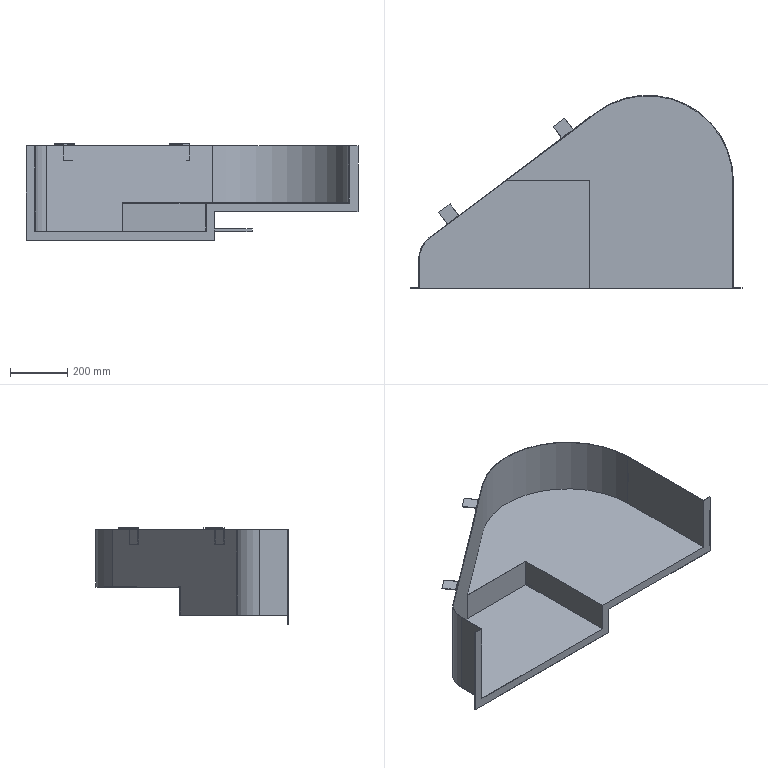Part | SolidWorks | features ICE 5, Extrusion 1, Shell 1 | 4 solids | 48 faces | box 1160 x 675 x 337 mm | volume 2407556 mm3 | plane 44 | cylinder 4 | commonest cylinder face diameters 196 x1 200 x1 596 x1 600 x1
STEP:
#1=CARTESIAN_POINT('',(-2.,0.,0.));
#2=VERTEX_POINT('',#1);
#3=CARTESIAN_POINT('',(30.,0.,0.));
#4=VERTEX_POINT('',#3);
#5=CARTESIAN_POINT('',(-1100.,0.,0.));
#6=DIRECTION('',(1.,0.,0.));
#7=VECTOR('',#6,1000.);
#8=LINE('',#5,#7);
#9=EDGE_CURVE('',#2,#4,#8,.T.);
#10=ORIENTED_EDGE('',*,*,#9,.F.);
#11=CARTESIAN_POINT('',(-2.,0.,-198.));
#12=VERTEX_POINT('',#11);
#13=CARTESIAN_POINT('',(-2.,0.,0.));
#14=DIRECTION('',(0.,0.,-1.));
#15=VECTOR('',#14,1000.);
#16=LINE('',#13,#15);
#17=EDGE_CURVE('',#2,#12,#16,.T.);
#18=ORIENTED_EDGE('',*,*,#17,.T.);
#19=CARTESIAN_POINT('',(-502.,0.,-198.));
#20=VERTEX_POINT('',#19);
#21=CARTESIAN_POINT('',(-1000.,0.,-198.));
#22=DIRECTION('',(-1.,0.,0.));
#23=VECTOR('',#22,1000.);
#24=LINE('',#21,#23);
#25=EDGE_CURVE('',#12,#20,#24,.T.);
#26=ORIENTED_EDGE('',*,*,#25,.T.);
#27=CARTESIAN_POINT('',(-502.,0.,-298.));
#28=VERTEX_POINT('',#27);
#29=CARTESIAN_POINT('',(-502.,0.,-300.));
#30=DIRECTION('',(0.,0.,-1.));
#31=VECTOR('',#30,1000.);
#32=LINE('',#29,#31);
#33=EDGE_CURVE('',#20,#28,#32,.T.);
#34=ORIENTED_EDGE('',*,*,#33,.T.);
#35=CARTESIAN_POINT('',(-1098.,0.,-298.));
#36=VERTEX_POINT('',#35);
#37=CARTESIAN_POINT('',(0.,0.,-298.));
#38=DIRECTION('',(-1.,0.,0.));
#39=VECTOR('',#38,1000.);
#40=LINE('',#37,#39);
#41=EDGE_CURVE('',#28,#36,#40,.T.);
#42=ORIENTED_EDGE('',*,*,#41,.T.);
#43=CARTESIAN_POINT('',(-1098.,0.,0.));
#44=VERTEX_POINT('',#43);
#45=CARTESIAN_POINT('',(-1098.,0.,0.));
#46=DIRECTION('',(0.,0.,1.));
#47=VECTOR('',#46,1000.);
#48=LINE('',#45,#47);
#49=EDGE_CURVE('',#36,#44,#48,.T.);
#50=ORIENTED_EDGE('',*,*,#49,.T.);
#51=CARTESIAN_POINT('',(-1130.,0.,0.));
#52=VERTEX_POINT('',#51);
#53=CARTESIAN_POINT('',(-1100.,0.,0.));
#54=DIRECTION('',(1.,0.,0.));
#55=VECTOR('',#54,1000.);
#56=LINE('',#53,#55);
#57=EDGE_CURVE('',#52,#44,#56,.T.);
#58=ORIENTED_EDGE('',*,*,#57,.F.);
#59=CARTESIAN_POINT('',(-1130.,0.,-330.));
#60=VERTEX_POINT('',#59);
#61=CARTESIAN_POINT('',(-1130.,0.,0.));
#62=DIRECTION('',(0.,0.,-1.));
#63=VECTOR('',#62,1000.);
#64=LINE('',#61,#63);
#65=EDGE_CURVE('',#52,#60,#64,.T.);
#66=ORIENTED_EDGE('',*,*,#65,.T.);
#67=CARTESIAN_POINT('',(-470.,0.,-330.));
#68=VERTEX_POINT('',#67);
#69=CARTESIAN_POINT('',(-1130.,0.,-330.));
#70=DIRECTION('',(1.,0.,0.));
#71=VECTOR('',#70,1000.);
#72=LINE('',#69,#71);
#73=EDGE_CURVE('',#60,#68,#72,.T.);
#74=ORIENTED_EDGE('',*,*,#73,.T.);
#75=CARTESIAN_POINT('',(-470.,0.,-230.));
#76=VERTEX_POINT('',#75);
#77=CARTESIAN_POINT('',(-470.,0.,-330.));
#78=DIRECTION('',(0.,0.,1.));
#79=VECTOR('',#78,1000.);
#80=LINE('',#77,#79);
#81=EDGE_CURVE('',#68,#76,#80,.T.);
#82=ORIENTED_EDGE('',*,*,#81,.T.);
#83=CARTESIAN_POINT('',(30.,0.,-230.));
#84=VERTEX_POINT('',#83);
#85=CARTESIAN_POINT('',(-470.,0.,-230.));
#86=DIRECTION('',(1.,0.,0.));
#87=VECTOR('',#86,1000.);
#88=LINE('',#85,#87);
#89=EDGE_CURVE('',#76,#84,#88,.T.);
#90=ORIENTED_EDGE('',*,*,#89,.T.);
#91=CARTESIAN_POINT('',(30.,0.,-230.));
#92=DIRECTION('',(0.,0.,1.));
#93=VECTOR('',#92,1000.);
#94=LINE('',#91,#93);
#95=EDGE_CURVE('',#84,#4,#94,.T.);
#96=ORIENTED_EDGE('',*,*,#95,.T.);
#97=EDGE_LOOP('',(#10,#18,#26,#34,#42,#50,#58,#66,#74,#82,#90,#96));
#98=FACE_OUTER_BOUND('',#97,.T.);
#99=CARTESIAN_POINT('',(-1100.,0.,-200.));
#100=DIRECTION('',(0.,-1.,0.));
#101=DIRECTION('',(0.,0.,-1.));
#102=AXIS2_PLACEMENT_3D('',#99,#100,#101);
#103=PLANE('',#102);
#104=ADVANCED_FACE('',(#98),#103,.T.);
#105=CARTESIAN_POINT('',(0.,2.,-200.));
#106=VERTEX_POINT('',#105);
#107=CARTESIAN_POINT('',(0.,375.,-200.));
#108=VERTEX_POINT('',#107);
#109=CARTESIAN_POINT('',(0.,0.,-200.));
#110=DIRECTION('',(0.,1.,0.));
#111=VECTOR('',#110,1000.);
#112=LINE('',#109,#111);
#113=EDGE_CURVE('',#106,#108,#112,.T.);
#114=ORIENTED_EDGE('',*,*,#113,.F.);
#115=CARTESIAN_POINT('',(-500.,2.,-200.));
#116=VERTEX_POINT('',#115);
#117=CARTESIAN_POINT('',(-500.,2.,-200.));
#118=DIRECTION('',(-1.,0.,0.));
#119=VECTOR('',#118,1000.);
#120=LINE('',#117,#119);
#121=EDGE_CURVE('',#106,#116,#120,.T.);
#122=ORIENTED_EDGE('',*,*,#121,.T.);
#123=CARTESIAN_POINT('',(-500.,380.,-200.));
#124=VERTEX_POINT('',#123);
#125=CARTESIAN_POINT('',(-500.,380.,-200.));
#126=DIRECTION('',(0.,-1.,0.));
#127=VECTOR('',#126,1000.);
#128=LINE('',#125,#127);
#129=EDGE_CURVE('',#124,#116,#128,.T.);
#130=ORIENTED_EDGE('',*,*,#129,.F.);
#131=CARTESIAN_POINT('',(-793.333,380.,-200.));
#132=VERTEX_POINT('',#131);
#133=CARTESIAN_POINT('',(-793.333,380.,-200.));
#134=DIRECTION('',(1.,0.,0.));
#135=VECTOR('',#134,1000.);
#136=LINE('',#133,#135);
#137=EDGE_CURVE('',#132,#124,#136,.T.);
#138=ORIENTED_EDGE('',*,*,#137,.F.);
#139=CARTESIAN_POINT('',(-480.,615.,-200.));
#140=VERTEX_POINT('',#139);
#141=CARTESIAN_POINT('',(-1060.,180.,-200.));
#142=DIRECTION('',(-0.8,-0.6,0.));
#143=VECTOR('',#142,1000.);
#144=LINE('',#141,#143);
#145=EDGE_CURVE('',#140,#132,#144,.T.);
#146=ORIENTED_EDGE('',*,*,#145,.F.);
#147=CARTESIAN_POINT('',(-300.,375.,-200.));
#148=DIRECTION('',(0.,0.,1.));
#149=DIRECTION('',(1.,0.,0.));
#150=AXIS2_PLACEMENT_3D('',#147,#148,#149);
#151=CIRCLE('',#150,300.);
#152=EDGE_CURVE('',#108,#140,#151,.T.);
#153=ORIENTED_EDGE('',*,*,#152,.F.);
#154=EDGE_LOOP('',(#114,#122,#130,#138,#146,#153));
#155=FACE_OUTER_BOUND('',#154,.T.);
#156=CARTESIAN_POINT('',(-1000.,100.,-200.));
#157=DIRECTION('',(0.,0.,1.));
#158=DIRECTION('',(1.,0.,0.));
#159=AXIS2_PLACEMENT_3D('',#156,#157,#158);
#160=PLANE('',#159);
#161=ADVANCED_FACE('',(#155),#160,.F.);
#162=CARTESIAN_POINT('',(-1060.,180.,0.));
#163=VERTEX_POINT('',#162);
#164=CARTESIAN_POINT('',(-1100.,100.,0.));
#165=VERTEX_POINT('',#164);
#166=CARTESIAN_POINT('',(-1000.,100.,0.));
#167=DIRECTION('',(0.,0.,1.));
#168=DIRECTION('',(1.,0.,0.));
#169=AXIS2_PLACEMENT_3D('',#166,#167,#168);
#170=CIRCLE('',#169,100.);
#171=EDGE_CURVE('',#163,#165,#170,.T.);
#172=ORIENTED_EDGE('',*,*,#171,.F.);
#173=CARTESIAN_POINT('',(-1060.,180.,-300.));
#174=VERTEX_POINT('',#173);
#175=CARTESIAN_POINT('',(-1060.,180.,-200.));
#176=DIRECTION('',(0.,0.,1.));
#177=VECTOR('',#176,1000.);
#178=LINE('',#175,#177);
#179=EDGE_CURVE('',#174,#163,#178,.T.);
#180=ORIENTED_EDGE('',*,*,#179,.F.);
#181=CARTESIAN_POINT('',(-1100.,100.,-300.));
#182=VERTEX_POINT('',#181);
#183=CARTESIAN_POINT('',(-1000.,100.,-300.));
#184=DIRECTION('',(0.,0.,-1.));
#185=DIRECTION('',(-1.,0.,0.));
#186=AXIS2_PLACEMENT_3D('',#183,#184,#185);
#187=CIRCLE('',#186,100.);
#188=EDGE_CURVE('',#182,#174,#187,.T.);
#189=ORIENTED_EDGE('',*,*,#188,.F.);
#190=CARTESIAN_POINT('',(-1100.,100.,-200.));
#191=DIRECTION('',(0.,0.,1.));
#192=VECTOR('',#191,1000.);
#193=LINE('',#190,#192);
#194=EDGE_CURVE('',#182,#165,#193,.T.);
#195=ORIENTED_EDGE('',*,*,#194,.T.);
#196=EDGE_LOOP('',(#172,#180,#189,#195));
#197=FACE_OUTER_BOUND('',#196,.T.);
#198=CARTESIAN_POINT('',(-1000.,100.,-200.));
#199=DIRECTION('',(0.,0.,1.));
#200=DIRECTION('',(1.,0.,0.));
#201=AXIS2_PLACEMENT_3D('',#198,#199,#200);
#202=CYLINDRICAL_SURFACE('',#201,100.);
#203=ADVANCED_FACE('',(#197),#202,.T.);
#204=CARTESIAN_POINT('',(-480.,615.,0.));
#205=VERTEX_POINT('',#204);
#206=CARTESIAN_POINT('',(-1060.,180.,0.));
#207=DIRECTION('',(-0.8,-0.6,0.));
#208=VECTOR('',#207,1000.);
#209=LINE('',#206,#208);
#210=EDGE_CURVE('',#205,#163,#209,.T.);
#211=ORIENTED_EDGE('',*,*,#210,.F.);
#212=CARTESIAN_POINT('',(-480.,615.,-200.));
#213=DIRECTION('',(0.,0.,1.));
#214=VECTOR('',#213,1000.);
#215=LINE('',#212,#214);
#216=EDGE_CURVE('',#140,#205,#215,.T.);
#217=ORIENTED_EDGE('',*,*,#216,.F.);
#218=ORIENTED_EDGE('',*,*,#145,.T.);
#219=CARTESIAN_POINT('',(-793.333,380.,-300.));
#220=VERTEX_POINT('',#219);
#221=CARTESIAN_POINT('',(-793.333,380.,-300.));
#222=DIRECTION('',(0.,0.,1.));
#223=VECTOR('',#222,1000.);
#224=LINE('',#221,#223);
#225=EDGE_CURVE('',#220,#132,#224,.T.);
#226=ORIENTED_EDGE('',*,*,#225,.F.);
#227=CARTESIAN_POINT('',(-793.333,380.,-300.));
#228=DIRECTION('',(0.8,0.6,0.));
#229=VECTOR('',#228,1000.);
#230=LINE('',#227,#229);
#231=EDGE_CURVE('',#174,#220,#230,.T.);
#232=ORIENTED_EDGE('',*,*,#231,.F.);
#233=ORIENTED_EDGE('',*,*,#179,.T.);
#234=EDGE_LOOP('',(#211,#217,#218,#226,#232,#233));
#235=FACE_OUTER_BOUND('',#234,.T.);
#236=CARTESIAN_POINT('',(-1060.,180.,-200.));
#237=DIRECTION('',(-0.6,0.8,0.));
#238=DIRECTION('',(-0.8,-0.6,0.));
#239=AXIS2_PLACEMENT_3D('',#236,#237,#238);
#240=PLANE('',#239);
#241=ADVANCED_FACE('',(#235),#240,.T.);
#242=CARTESIAN_POINT('',(0.,375.,0.));
#243=VERTEX_POINT('',#242);
#244=CARTESIAN_POINT('',(-300.,375.,0.));
#245=DIRECTION('',(0.,0.,1.));
#246=DIRECTION('',(1.,0.,0.));
#247=AXIS2_PLACEMENT_3D('',#244,#245,#246);
#248=CIRCLE('',#247,300.);
#249=EDGE_CURVE('',#243,#205,#248,.T.);
#250=ORIENTED_EDGE('',*,*,#249,.F.);
#251=CARTESIAN_POINT('',(0.,375.,-200.));
#252=DIRECTION('',(0.,0.,1.));
#253=VECTOR('',#252,1000.);
#254=LINE('',#251,#253);
#255=EDGE_CURVE('',#108,#243,#254,.T.);
#256=ORIENTED_EDGE('',*,*,#255,.F.);
#257=ORIENTED_EDGE('',*,*,#152,.T.);
#258=ORIENTED_EDGE('',*,*,#216,.T.);
#259=EDGE_LOOP('',(#250,#256,#257,#258));
#260=FACE_OUTER_BOUND('',#259,.T.);
#261=CARTESIAN_POINT('',(-300.,375.,-200.));
#262=DIRECTION('',(0.,0.,1.));
#263=DIRECTION('',(1.,0.,0.));
#264=AXIS2_PLACEMENT_3D('',#261,#262,#263);
#265=CYLINDRICAL_SURFACE('',#264,300.);
#266=ADVANCED_FACE('',(#260),#265,.T.);
#267=CARTESIAN_POINT('',(0.,2.,0.));
#268=VERTEX_POINT('',#267);
#269=CARTESIAN_POINT('',(0.,2.,-200.));
#270=DIRECTION('',(0.,0.,-1.));
#271=VECTOR('',#270,1000.);
#272=LINE('',#269,#271);
#273=EDGE_CURVE('',#268,#106,#272,.T.);
#274=ORIENTED_EDGE('',*,*,#273,.T.);
#275=ORIENTED_EDGE('',*,*,#113,.T.);
#276=ORIENTED_EDGE('',*,*,#255,.T.);
#277=CARTESIAN_POINT('',(0.,0.,0.));
#278=DIRECTION('',(0.,1.,0.));
#279=VECTOR('',#278,1000.);
#280=LINE('',#277,#279);
#281=EDGE_CURVE('',#268,#243,#280,.T.);
#282=ORIENTED_EDGE('',*,*,#281,.F.);
#283=EDGE_LOOP('',(#274,#275,#276,#282));
#284=FACE_OUTER_BOUND('',#283,.T.);
#285=CARTESIAN_POINT('',(0.,0.,-200.));
#286=DIRECTION('',(1.,0.,0.));
#287=DIRECTION('',(0.,0.,-1.));
#288=AXIS2_PLACEMENT_3D('',#285,#286,#287);
#289=PLANE('',#288);
#290=ADVANCED_FACE('',(#284),#289,.T.);
#291=CARTESIAN_POINT('',(-1100.,2.,-300.));
#292=VERTEX_POINT('',#291);
#293=CARTESIAN_POINT('',(-1100.,2.,0.));
#294=VERTEX_POINT('',#293);
#295=CARTESIAN_POINT('',(-1100.,2.,0.));
#296=DIRECTION('',(0.,0.,1.));
#297=VECTOR('',#296,1000.);
#298=LINE('',#295,#297);
#299=EDGE_CURVE('',#292,#294,#298,.T.);
#300=ORIENTED_EDGE('',*,*,#299,.T.);
#301=CARTESIAN_POINT('',(-1100.,100.,0.));
#302=DIRECTION('',(0.,-1.,0.));
#303=VECTOR('',#302,1000.);
#304=LINE('',#301,#303);
#305=EDGE_CURVE('',#165,#294,#304,.T.);
#306=ORIENTED_EDGE('',*,*,#305,.F.);
#307=ORIENTED_EDGE('',*,*,#194,.F.);
#308=CARTESIAN_POINT('',(-1100.,100.,-300.));
#309=DIRECTION('',(0.,1.,0.));
#310=VECTOR('',#309,1000.);
#311=LINE('',#308,#310);
#312=EDGE_CURVE('',#292,#182,#311,.T.);
#313=ORIENTED_EDGE('',*,*,#312,.F.);
#314=EDGE_LOOP('',(#300,#306,#307,#313));
#315=FACE_OUTER_BOUND('',#314,.T.);
#316=CARTESIAN_POINT('',(-1100.,100.,-200.));
#317=DIRECTION('',(-1.,0.,0.));
#318=DIRECTION('',(0.,0.,1.));
#319=AXIS2_PLACEMENT_3D('',#316,#317,#318);
#320=PLANE('',#319);
#321=ADVANCED_FACE('',(#315),#320,.T.);
#322=CARTESIAN_POINT('',(-1098.,100.,0.));
#323=VERTEX_POINT('',#322);
#324=CARTESIAN_POINT('',(-1098.,100.,0.));
#325=DIRECTION('',(0.,-1.,0.));
#326=VECTOR('',#325,1000.);
#327=LINE('',#324,#326);
#328=EDGE_CURVE('',#323,#44,#327,.T.);
#329=ORIENTED_EDGE('',*,*,#328,.F.);
#330=CARTESIAN_POINT('',(-1058.8,178.4,0.));
#331=VERTEX_POINT('',#330);
#332=CARTESIAN_POINT('',(-1000.,100.,0.));
#333=DIRECTION('',(0.,0.,1.));
#334=DIRECTION('',(1.,0.,0.));
#335=AXIS2_PLACEMENT_3D('',#332,#333,#334);
#336=CIRCLE('',#335,98.);
#337=EDGE_CURVE('',#331,#323,#336,.T.);
#338=ORIENTED_EDGE('',*,*,#337,.F.);
#339=CARTESIAN_POINT('',(-478.8,613.4,0.));
#340=VERTEX_POINT('',#339);
#341=CARTESIAN_POINT('',(-1058.8,178.4,0.));
#342=DIRECTION('',(-0.8,-0.6,0.));
#343=VECTOR('',#342,1000.);
#344=LINE('',#341,#343);
#345=EDGE_CURVE('',#340,#331,#344,.T.);
#346=ORIENTED_EDGE('',*,*,#345,.F.);
#347=CARTESIAN_POINT('',(-2.,375.,0.));
#348=VERTEX_POINT('',#347);
#349=CARTESIAN_POINT('',(-300.,375.,0.));
#350=DIRECTION('',(0.,0.,1.));
#351=DIRECTION('',(1.,0.,0.));
#352=AXIS2_PLACEMENT_3D('',#349,#350,#351);
#353=CIRCLE('',#352,298.);
#354=EDGE_CURVE('',#348,#340,#353,.T.);
#355=ORIENTED_EDGE('',*,*,#354,.F.);
#356=CARTESIAN_POINT('',(-2.,100.,0.));
#357=DIRECTION('',(0.,1.,0.));
#358=VECTOR('',#357,1000.);
#359=LINE('',#356,#358);
#360=EDGE_CURVE('',#2,#348,#359,.T.);
#361=ORIENTED_EDGE('',*,*,#360,.F.);
#362=ORIENTED_EDGE('',*,*,#9,.T.);
#363=CARTESIAN_POINT('',(30.,2.,0.));
#364=VERTEX_POINT('',#363);
#365=CARTESIAN_POINT('',(30.,2.,0.));
#366=DIRECTION('',(0.,-1.,0.));
#367=VECTOR('',#366,1000.);
#368=LINE('',#365,#367);
#369=EDGE_CURVE('',#364,#4,#368,.T.);
#370=ORIENTED_EDGE('',*,*,#369,.F.);
#371=CARTESIAN_POINT('',(30.,2.,0.));
#372=DIRECTION('',(-1.,0.,0.));
#373=VECTOR('',#372,1000.);
#374=LINE('',#371,#373);
#375=EDGE_CURVE('',#364,#268,#374,.T.);
#376=ORIENTED_EDGE('',*,*,#375,.T.);
#377=ORIENTED_EDGE('',*,*,#281,.T.);
#378=ORIENTED_EDGE('',*,*,#249,.T.);
#379=ORIENTED_EDGE('',*,*,#210,.T.);
#380=ORIENTED_EDGE('',*,*,#171,.T.);
#381=ORIENTED_EDGE('',*,*,#305,.T.);
#382=CARTESIAN_POINT('',(-1130.,2.,0.));
#383=VERTEX_POINT('',#382);
#384=CARTESIAN_POINT('',(-1100.,2.,0.));
#385=DIRECTION('',(-1.,0.,0.));
#386=VECTOR('',#385,1000.);
#387=LINE('',#384,#386);
#388=EDGE_CURVE('',#294,#383,#387,.T.);
#389=ORIENTED_EDGE('',*,*,#388,.T.);
#390=CARTESIAN_POINT('',(-1130.,2.,0.));
#391=DIRECTION('',(0.,-1.,0.));
#392=VECTOR('',#391,1000.);
#393=LINE('',#390,#392);
#394=EDGE_CURVE('',#383,#52,#393,.T.);
#395=ORIENTED_EDGE('',*,*,#394,.T.);
#396=ORIENTED_EDGE('',*,*,#57,.T.);
#397=EDGE_LOOP('',(#329,#338,#346,#355,#361,#362,#370,#376,#377,#378,#379,#380,#381,#389,#395,#396));
#398=FACE_OUTER_BOUND('',#397,.T.);
#399=CARTESIAN_POINT('',(-1000.,100.,0.));
#400=DIRECTION('',(0.,0.,1.));
#401=DIRECTION('',(1.,0.,0.));
#402=AXIS2_PLACEMENT_3D('',#399,#400,#401);
#403=PLANE('',#402);
#404=ADVANCED_FACE('',(#398),#403,.T.);
#405=ORIENTED_EDGE('',*,*,#137,.T.);
#406=CARTESIAN_POINT('',(-500.,380.,-300.));
#407=VERTEX_POINT('',#406);
#408=CARTESIAN_POINT('',(-500.,380.,-300.));
#409=DIRECTION('',(0.,0.,1.));
#410=VECTOR('',#409,1000.);
#411=LINE('',#408,#410);
#412=EDGE_CURVE('',#407,#124,#411,.T.);
#413=ORIENTED_EDGE('',*,*,#412,.F.);
#414=CARTESIAN_POINT('',(-793.333,380.,-300.));
#415=DIRECTION('',(1.,0.,0.));
#416=VECTOR('',#415,1000.);
#417=LINE('',#414,#416);
#418=EDGE_CURVE('',#220,#407,#417,.T.);
#419=ORIENTED_EDGE('',*,*,#418,.F.);
#420=ORIENTED_EDGE('',*,*,#225,.T.);
#421=EDGE_LOOP('',(#405,#413,#419,#420));
#422=FACE_OUTER_BOUND('',#421,.T.);
#423=CARTESIAN_POINT('',(-793.333,380.,-300.));
#424=DIRECTION('',(0.,-1.,0.));
#425=DIRECTION('',(1.,0.,0.));
#426=AXIS2_PLACEMENT_3D('',#423,#424,#425);
#427=PLANE('',#426);
#428=ADVANCED_FACE('',(#422),#427,.F.);
#429=ORIENTED_EDGE('',*,*,#129,.T.);
#430=CARTESIAN_POINT('',(-500.,2.,-300.));
#431=VERTEX_POINT('',#430);
#432=CARTESIAN_POINT('',(-500.,2.,-300.));
#433=DIRECTION('',(0.,0.,-1.));
#434=VECTOR('',#433,1000.);
#435=LINE('',#432,#434);
#436=EDGE_CURVE('',#116,#431,#435,.T.);
#437=ORIENTED_EDGE('',*,*,#436,.T.);
#438=CARTESIAN_POINT('',(-500.,380.,-300.));
#439=DIRECTION('',(0.,-1.,0.));
#440=VECTOR('',#439,1000.);
#441=LINE('',#438,#440);
#442=EDGE_CURVE('',#407,#431,#441,.T.);
#443=ORIENTED_EDGE('',*,*,#442,.F.);
#444=ORIENTED_EDGE('',*,*,#412,.T.);
#445=EDGE_LOOP('',(#429,#437,#443,#444));
#446=FACE_OUTER_BOUND('',#445,.T.);
#447=CARTESIAN_POINT('',(-500.,380.,-300.));
#448=DIRECTION('',(-1.,0.,0.));
#449=DIRECTION('',(0.,0.,1.));
#450=AXIS2_PLACEMENT_3D('',#447,#448,#449);
#451=PLANE('',#450);
#452=ADVANCED_FACE('',(#446),#451,.F.);
#453=CARTESIAN_POINT('',(-1100.,2.,-300.));
#454=DIRECTION('',(-1.,0.,0.));
#455=VECTOR('',#454,1000.);
#456=LINE('',#453,#455);
#457=EDGE_CURVE('',#431,#292,#456,.T.);
#458=ORIENTED_EDGE('',*,*,#457,.T.);
#459=ORIENTED_EDGE('',*,*,#312,.T.);
#460=ORIENTED_EDGE('',*,*,#188,.T.);
#461=ORIENTED_EDGE('',*,*,#231,.T.);
#462=ORIENTED_EDGE('',*,*,#418,.T.);
#463=ORIENTED_EDGE('',*,*,#442,.T.);
#464=EDGE_LOOP('',(#458,#459,#460,#461,#462,#463));
#465=FACE_OUTER_BOUND('',#464,.T.);
#466=CARTESIAN_POINT('',(-1000.,100.,-300.));
#467=DIRECTION('',(0.,0.,-1.));
#468=DIRECTION('',(-1.,0.,0.));
#469=AXIS2_PLACEMENT_3D('',#466,#467,#468);
#470=PLANE('',#469);
#471=ADVANCED_FACE('',(#465),#470,.T.);
#472=ORIENTED_EDGE('',*,*,#95,.F.);
#473=CARTESIAN_POINT('',(30.,2.,-230.));
#474=VERTEX_POINT('',#473);
#475=CARTESIAN_POINT('',(30.,2.,-230.));
#476=DIRECTION('',(0.,-1.,0.));
#477=VECTOR('',#476,1000.);
#478=LINE('',#475,#477);
#479=EDGE_CURVE('',#474,#84,#478,.T.);
#480=ORIENTED_EDGE('',*,*,#479,.F.);
#481=CARTESIAN_POINT('',(30.,2.,-230.));
#482=DIRECTION('',(0.,0.,1.));
#483=VECTOR('',#482,1000.);
#484=LINE('',#481,#483);
#485=EDGE_CURVE('',#474,#364,#484,.T.);
#486=ORIENTED_EDGE('',*,*,#485,.T.);
#487=ORIENTED_EDGE('',*,*,#369,.T.);
#488=EDGE_LOOP('',(#472,#480,#486,#487));
#489=FACE_OUTER_BOUND('',#488,.T.);
#490=CARTESIAN_POINT('',(30.,2.,-230.));
#491=DIRECTION('',(1.,0.,0.));
#492=DIRECTION('',(0.,0.,-1.));
#493=AXIS2_PLACEMENT_3D('',#490,#491,#492);
#494=PLANE('',#493);
#495=ADVANCED_FACE('',(#489),#494,.T.);
#496=ORIENTED_EDGE('',*,*,#89,.F.);
#497=CARTESIAN_POINT('',(-470.,2.,-230.));
#498=VERTEX_POINT('',#497);
#499=CARTESIAN_POINT('',(-470.,2.,-230.));
#500=DIRECTION('',(0.,-1.,0.));
#501=VECTOR('',#500,1000.);
#502=LINE('',#499,#501);
#503=EDGE_CURVE('',#498,#76,#502,.T.);
#504=ORIENTED_EDGE('',*,*,#503,.F.);
#505=CARTESIAN_POINT('',(-470.,2.,-230.));
#506=DIRECTION('',(1.,0.,0.));
#507=VECTOR('',#506,1000.);
#508=LINE('',#505,#507);
#509=EDGE_CURVE('',#498,#474,#508,.T.);
#510=ORIENTED_EDGE('',*,*,#509,.T.);
#511=ORIENTED_EDGE('',*,*,#479,.T.);
#512=EDGE_LOOP('',(#496,#504,#510,#511));
#513=FACE_OUTER_BOUND('',#512,.T.);
#514=CARTESIAN_POINT('',(-470.,2.,-230.));
#515=DIRECTION('',(0.,0.,-1.));
#516=DIRECTION('',(-1.,0.,0.));
#517=AXIS2_PLACEMENT_3D('',#514,#515,#516);
#518=PLANE('',#517);
#519=ADVANCED_FACE('',(#513),#518,.T.);
#520=ORIENTED_EDGE('',*,*,#81,.F.);
#521=CARTESIAN_POINT('',(-470.,2.,-330.));
#522=VERTEX_POINT('',#521);
#523=CARTESIAN_POINT('',(-470.,2.,-330.));
#524=DIRECTION('',(0.,-1.,0.));
#525=VECTOR('',#524,1000.);
#526=LINE('',#523,#525);
#527=EDGE_CURVE('',#522,#68,#526,.T.);
#528=ORIENTED_EDGE('',*,*,#527,.F.);
#529=CARTESIAN_POINT('',(-470.,2.,-330.));
#530=DIRECTION('',(0.,0.,1.));
#531=VECTOR('',#530,1000.);
#532=LINE('',#529,#531);
#533=EDGE_CURVE('',#522,#498,#532,.T.);
#534=ORIENTED_EDGE('',*,*,#533,.T.);
#535=ORIENTED_EDGE('',*,*,#503,.T.);
#536=EDGE_LOOP('',(#520,#528,#534,#535));
#537=FACE_OUTER_BOUND('',#536,.T.);
#538=CARTESIAN_POINT('',(-470.,2.,-330.));
#539=DIRECTION('',(1.,0.,0.));
#540=DIRECTION('',(0.,0.,-1.));
#541=AXIS2_PLACEMENT_3D('',#538,#539,#540);
#542=PLANE('',#541);
#543=ADVANCED_FACE('',(#537),#542,.T.);
#544=ORIENTED_EDGE('',*,*,#73,.F.);
#545=CARTESIAN_POINT('',(-1130.,2.,-330.));
#546=VERTEX_POINT('',#545);
#547=CARTESIAN_POINT('',(-1130.,2.,-330.));
#548=DIRECTION('',(0.,-1.,0.));
#549=VECTOR('',#548,1000.);
#550=LINE('',#547,#549);
#551=EDGE_CURVE('',#546,#60,#550,.T.);
#552=ORIENTED_EDGE('',*,*,#551,.F.);
#553=CARTESIAN_POINT('',(-1130.,2.,-330.));
#554=DIRECTION('',(1.,0.,0.));
#555=VECTOR('',#554,1000.);
#556=LINE('',#553,#555);
#557=EDGE_CURVE('',#546,#522,#556,.T.);
#558=ORIENTED_EDGE('',*,*,#557,.T.);
#559=ORIENTED_EDGE('',*,*,#527,.T.);
#560=EDGE_LOOP('',(#544,#552,#558,#559));
#561=FACE_OUTER_BOUND('',#560,.T.);
#562=CARTESIAN_POINT('',(-1130.,2.,-330.));
#563=DIRECTION('',(0.,0.,-1.));
#564=DIRECTION('',(-1.,0.,0.));
#565=AXIS2_PLACEMENT_3D('',#562,#563,#564);
#566=PLANE('',#565);
#567=ADVANCED_FACE('',(#561),#566,.T.);
#568=ORIENTED_EDGE('',*,*,#65,.F.);
#569=ORIENTED_EDGE('',*,*,#394,.F.);
#570=CARTESIAN_POINT('',(-1130.,2.,0.));
#571=DIRECTION('',(0.,0.,-1.));
#572=VECTOR('',#571,1000.);
#573=LINE('',#570,#572);
#574=EDGE_CURVE('',#383,#546,#573,.T.);
#575=ORIENTED_EDGE('',*,*,#574,.T.);
#576=ORIENTED_EDGE('',*,*,#551,.T.);
#577=EDGE_LOOP('',(#568,#569,#575,#576));
#578=FACE_OUTER_BOUND('',#577,.T.);
#579=CARTESIAN_POINT('',(-1130.,2.,0.));
#580=DIRECTION('',(-1.,0.,0.));
#581=DIRECTION('',(0.,0.,1.));
#582=AXIS2_PLACEMENT_3D('',#579,#580,#581);
#583=PLANE('',#582);
#584=ADVANCED_FACE('',(#578),#583,.T.);
#585=ORIENTED_EDGE('',*,*,#375,.F.);
#586=ORIENTED_EDGE('',*,*,#485,.F.);
#587=ORIENTED_EDGE('',*,*,#509,.F.);
#588=ORIENTED_EDGE('',*,*,#533,.F.);
#589=ORIENTED_EDGE('',*,*,#557,.F.);
#590=ORIENTED_EDGE('',*,*,#574,.F.);
#591=ORIENTED_EDGE('',*,*,#388,.F.);
#592=ORIENTED_EDGE('',*,*,#299,.F.);
#593=ORIENTED_EDGE('',*,*,#457,.F.);
#594=ORIENTED_EDGE('',*,*,#436,.F.);
#595=ORIENTED_EDGE('',*,*,#121,.F.);
#596=ORIENTED_EDGE('',*,*,#273,.F.);
#597=EDGE_LOOP('',(#585,#586,#587,#588,#589,#590,#591,#592,#593,#594,#595,#596));
#598=FACE_OUTER_BOUND('',#597,.T.);
#599=CARTESIAN_POINT('',(0.,2.,0.));
#600=DIRECTION('',(0.,1.,0.));
#601=DIRECTION('',(0.,0.,1.));
#602=AXIS2_PLACEMENT_3D('',#599,#600,#601);
#603=PLANE('',#602);
#604=ADVANCED_FACE('',(#598),#603,.T.);
#605=CARTESIAN_POINT('',(-2.,375.,-198.));
#606=VERTEX_POINT('',#605);
#607=CARTESIAN_POINT('',(-2.,100.,-198.));
#608=DIRECTION('',(0.,1.,0.));
#609=VECTOR('',#608,1000.);
#610=LINE('',#607,#609);
#611=EDGE_CURVE('',#12,#606,#610,.T.);
#612=ORIENTED_EDGE('',*,*,#611,.T.);
#613=CARTESIAN_POINT('',(-478.8,613.4,-198.));
#614=VERTEX_POINT('',#613);
#615=CARTESIAN_POINT('',(-300.,375.,-198.));
#616=DIRECTION('',(0.,0.,1.));
#617=DIRECTION('',(1.,0.,0.));
#618=AXIS2_PLACEMENT_3D('',#615,#616,#617);
#619=CIRCLE('',#618,298.);
#620=EDGE_CURVE('',#606,#614,#619,.T.);
#621=ORIENTED_EDGE('',*,*,#620,.T.);
#622=CARTESIAN_POINT('',(-792.667,378.,-198.));
#623=VERTEX_POINT('',#622);
#624=CARTESIAN_POINT('',(-1058.8,178.4,-198.));
#625=DIRECTION('',(-0.8,-0.6,0.));
#626=VECTOR('',#625,1000.);
#627=LINE('',#624,#626);
#628=EDGE_CURVE('',#614,#623,#627,.T.);
#629=ORIENTED_EDGE('',*,*,#628,.T.);
#630=CARTESIAN_POINT('',(-502.,378.,-198.));
#631=VERTEX_POINT('',#630);
#632=CARTESIAN_POINT('',(-1000.,378.,-198.));
#633=DIRECTION('',(1.,0.,0.));
#634=VECTOR('',#633,1000.);
#635=LINE('',#632,#634);
#636=EDGE_CURVE('',#623,#631,#635,.T.);
#637=ORIENTED_EDGE('',*,*,#636,.T.);
#638=CARTESIAN_POINT('',(-502.,100.,-198.));
#639=DIRECTION('',(0.,-1.,0.));
#640=VECTOR('',#639,1000.);
#641=LINE('',#638,#640);
#642=EDGE_CURVE('',#631,#20,#641,.T.);
#643=ORIENTED_EDGE('',*,*,#642,.T.);
#644=ORIENTED_EDGE('',*,*,#25,.F.);
#645=EDGE_LOOP('',(#612,#621,#629,#637,#643,#644));
#646=FACE_OUTER_BOUND('',#645,.T.);
#647=CARTESIAN_POINT('',(-1000.,100.,-198.));
#648=DIRECTION('',(0.,0.,1.));
#649=DIRECTION('',(1.,0.,0.));
#650=AXIS2_PLACEMENT_3D('',#647,#648,#649);
#651=PLANE('',#650);
#652=ADVANCED_FACE('',(#646),#651,.T.);
#653=ORIENTED_EDGE('',*,*,#337,.T.);
#654=CARTESIAN_POINT('',(-1098.,100.,-298.));
#655=VERTEX_POINT('',#654);
#656=CARTESIAN_POINT('',(-1098.,100.,-200.));
#657=DIRECTION('',(0.,0.,1.));
#658=VECTOR('',#657,1000.);
#659=LINE('',#656,#658);
#660=EDGE_CURVE('',#655,#323,#659,.T.);
#661=ORIENTED_EDGE('',*,*,#660,.F.);
#662=CARTESIAN_POINT('',(-1058.8,178.4,-298.));
#663=VERTEX_POINT('',#662);
#664=CARTESIAN_POINT('',(-1000.,100.,-298.));
#665=DIRECTION('',(0.,0.,-1.));
#666=DIRECTION('',(-1.,0.,0.));
#667=AXIS2_PLACEMENT_3D('',#664,#665,#666);
#668=CIRCLE('',#667,98.);
#669=EDGE_CURVE('',#655,#663,#668,.T.);
#670=ORIENTED_EDGE('',*,*,#669,.T.);
#671=CARTESIAN_POINT('',(-1058.8,178.4,-200.));
#672=DIRECTION('',(0.,0.,1.));
#673=VECTOR('',#672,1000.);
#674=LINE('',#671,#673);
#675=EDGE_CURVE('',#663,#331,#674,.T.);
#676=ORIENTED_EDGE('',*,*,#675,.T.);
#677=EDGE_LOOP('',(#653,#661,#670,#676));
#678=FACE_OUTER_BOUND('',#677,.T.);
#679=CARTESIAN_POINT('',(-1000.,100.,-200.));
#680=DIRECTION('',(0.,0.,1.));
#681=DIRECTION('',(1.,0.,0.));
#682=AXIS2_PLACEMENT_3D('',#679,#680,#681);
#683=CYLINDRICAL_SURFACE('',#682,98.);
#684=ADVANCED_FACE('',(#678),#683,.F.);
#685=ORIENTED_EDGE('',*,*,#345,.T.);
#686=ORIENTED_EDGE('',*,*,#675,.F.);
#687=CARTESIAN_POINT('',(-792.667,378.,-298.));
#688=VERTEX_POINT('',#687);
#689=CARTESIAN_POINT('',(-1058.8,178.4,-298.));
#690=DIRECTION('',(0.8,0.6,0.));
#691=VECTOR('',#690,1000.);
#692=LINE('',#689,#691);
#693=EDGE_CURVE('',#663,#688,#692,.T.);
#694=ORIENTED_EDGE('',*,*,#693,.T.);
#695=CARTESIAN_POINT('',(-792.667,378.,-200.));
#696=DIRECTION('',(0.,0.,1.));
#697=VECTOR('',#696,1000.);
#698=LINE('',#695,#697);
#699=EDGE_CURVE('',#688,#623,#698,.T.);
#700=ORIENTED_EDGE('',*,*,#699,.T.);
#701=ORIENTED_EDGE('',*,*,#628,.F.);
#702=CARTESIAN_POINT('',(-478.8,613.4,-200.));
#703=DIRECTION('',(0.,0.,1.));
#704=VECTOR('',#703,1000.);
#705=LINE('',#702,#704);
#706=EDGE_CURVE('',#614,#340,#705,.T.);
#707=ORIENTED_EDGE('',*,*,#706,.T.);
#708=EDGE_LOOP('',(#685,#686,#694,#700,#701,#707));
#709=FACE_OUTER_BOUND('',#708,.T.);
#710=CARTESIAN_POINT('',(-1058.8,178.4,-200.));
#711=DIRECTION('',(-0.6,0.8,0.));
#712=DIRECTION('',(-0.8,-0.6,0.));
#713=AXIS2_PLACEMENT_3D('',#710,#711,#712);
#714=PLANE('',#713);
#715=ADVANCED_FACE('',(#709),#714,.F.);
#716=ORIENTED_EDGE('',*,*,#354,.T.);
#717=ORIENTED_EDGE('',*,*,#706,.F.);
#718=ORIENTED_EDGE('',*,*,#620,.F.);
#719=CARTESIAN_POINT('',(-2.,375.,-200.));
#720=DIRECTION('',(0.,0.,1.));
#721=VECTOR('',#720,1000.);
#722=LINE('',#719,#721);
#723=EDGE_CURVE('',#606,#348,#722,.T.);
#724=ORIENTED_EDGE('',*,*,#723,.T.);
#725=EDGE_LOOP('',(#716,#717,#718,#724));
#726=FACE_OUTER_BOUND('',#725,.T.);
#727=CARTESIAN_POINT('',(-300.,375.,-200.));
#728=DIRECTION('',(0.,0.,1.));
#729=DIRECTION('',(1.,0.,0.));
#730=AXIS2_PLACEMENT_3D('',#727,#728,#729);
#731=CYLINDRICAL_SURFACE('',#730,298.);
#732=ADVANCED_FACE('',(#726),#731,.F.);
#733=ORIENTED_EDGE('',*,*,#17,.F.);
#734=ORIENTED_EDGE('',*,*,#360,.T.);
#735=ORIENTED_EDGE('',*,*,#723,.F.);
#736=ORIENTED_EDGE('',*,*,#611,.F.);
#737=EDGE_LOOP('',(#733,#734,#735,#736));
#738=FACE_OUTER_BOUND('',#737,.T.);
#739=CARTESIAN_POINT('',(-2.,0.,-200.));
#740=DIRECTION('',(1.,0.,0.));
#741=DIRECTION('',(0.,0.,-1.));
#742=AXIS2_PLACEMENT_3D('',#739,#740,#741);
#743=PLANE('',#742);
#744=ADVANCED_FACE('',(#738),#743,.F.);
#745=ORIENTED_EDGE('',*,*,#49,.F.);
#746=CARTESIAN_POINT('',(-1098.,100.,-298.));
#747=DIRECTION('',(0.,1.,0.));
#748=VECTOR('',#747,1000.);
#749=LINE('',#746,#748);
#750=EDGE_CURVE('',#36,#655,#749,.T.);
#751=ORIENTED_EDGE('',*,*,#750,.T.);
#752=ORIENTED_EDGE('',*,*,#660,.T.);
#753=ORIENTED_EDGE('',*,*,#328,.T.);
#754=EDGE_LOOP('',(#745,#751,#752,#753));
#755=FACE_OUTER_BOUND('',#754,.T.);
#756=CARTESIAN_POINT('',(-1098.,100.,-200.));
#757=DIRECTION('',(-1.,0.,0.));
#758=DIRECTION('',(0.,0.,1.));
#759=AXIS2_PLACEMENT_3D('',#756,#757,#758);
#760=PLANE('',#759);
#761=ADVANCED_FACE('',(#755),#760,.F.);
#762=ORIENTED_EDGE('',*,*,#636,.F.);
#763=ORIENTED_EDGE('',*,*,#699,.F.);
#764=CARTESIAN_POINT('',(-502.,378.,-298.));
#765=VERTEX_POINT('',#764);
#766=CARTESIAN_POINT('',(-793.333,378.,-298.));
#767=DIRECTION('',(1.,0.,0.));
#768=VECTOR('',#767,1000.);
#769=LINE('',#766,#768);
#770=EDGE_CURVE('',#688,#765,#769,.T.);
#771=ORIENTED_EDGE('',*,*,#770,.T.);
#772=CARTESIAN_POINT('',(-502.,378.,-300.));
#773=DIRECTION('',(0.,0.,1.));
#774=VECTOR('',#773,1000.);
#775=LINE('',#772,#774);
#776=EDGE_CURVE('',#765,#631,#775,.T.);
#777=ORIENTED_EDGE('',*,*,#776,.T.);
#778=EDGE_LOOP('',(#762,#763,#771,#777));
#779=FACE_OUTER_BOUND('',#778,.T.);
#780=CARTESIAN_POINT('',(-793.333,378.,-300.));
#781=DIRECTION('',(0.,-1.,0.));
#782=DIRECTION('',(1.,0.,0.));
#783=AXIS2_PLACEMENT_3D('',#780,#781,#782);
#784=PLANE('',#783);
#785=ADVANCED_FACE('',(#779),#784,.T.);
#786=ORIENTED_EDGE('',*,*,#642,.F.);
#787=ORIENTED_EDGE('',*,*,#776,.F.);
#788=CARTESIAN_POINT('',(-502.,380.,-298.));
#789=DIRECTION('',(0.,-1.,0.));
#790=VECTOR('',#789,1000.);
#791=LINE('',#788,#790);
#792=EDGE_CURVE('',#765,#28,#791,.T.);
#793=ORIENTED_EDGE('',*,*,#792,.T.);
#794=ORIENTED_EDGE('',*,*,#33,.F.);
#795=EDGE_LOOP('',(#786,#787,#793,#794));
#796=FACE_OUTER_BOUND('',#795,.T.);
#797=CARTESIAN_POINT('',(-502.,380.,-300.));
#798=DIRECTION('',(-1.,0.,0.));
#799=DIRECTION('',(0.,0.,1.));
#800=AXIS2_PLACEMENT_3D('',#797,#798,#799);
#801=PLANE('',#800);
#802=ADVANCED_FACE('',(#796),#801,.T.);
#803=ORIENTED_EDGE('',*,*,#41,.F.);
#804=ORIENTED_EDGE('',*,*,#792,.F.);
#805=ORIENTED_EDGE('',*,*,#770,.F.);
#806=ORIENTED_EDGE('',*,*,#693,.F.);
#807=ORIENTED_EDGE('',*,*,#669,.F.);
#808=ORIENTED_EDGE('',*,*,#750,.F.);
#809=EDGE_LOOP('',(#803,#804,#805,#806,#807,#808));
#810=FACE_OUTER_BOUND('',#809,.T.);
#811=CARTESIAN_POINT('',(-1000.,100.,-298.));
#812=DIRECTION('',(0.,0.,-1.));
#813=DIRECTION('',(-1.,0.,0.));
#814=AXIS2_PLACEMENT_3D('',#811,#812,#813);
#815=PLANE('',#814);
#816=ADVANCED_FACE('',(#810),#815,.F.);
#817=CLOSED_SHELL('',(#104,#161,#203,#241,#266,#290,#321,#404,#428,#452,#471,#495,#519,#543,#567,#584,#604,#652,#684,#715,#732,#744,#761,#785,#802,#816));
#818=MANIFOLD_SOLID_BREP('',#817);
#819=CARTESIAN_POINT('',(-500.,260.,-300.));
#820=VERTEX_POINT('',#819);
#821=CARTESIAN_POINT('',(-500.,380.,-300.));
#822=VERTEX_POINT('',#821);
#823=CARTESIAN_POINT('',(-500.,380.,-300.));
#824=DIRECTION('',(0.,1.,0.));
#825=VECTOR('',#824,1000.);
#826=LINE('',#823,#825);
#827=EDGE_CURVE('',#820,#822,#826,.T.);
#828=ORIENTED_EDGE('',*,*,#827,.F.);
#829=CARTESIAN_POINT('',(-500.,260.,-290.));
#830=VERTEX_POINT('',#829);
#831=CARTESIAN_POINT('',(-500.,260.,-290.));
#832=DIRECTION('',(0.,0.,-1.));
#833=VECTOR('',#832,1000.);
#834=LINE('',#831,#833);
#835=EDGE_CURVE('',#830,#820,#834,.T.);
#836=ORIENTED_EDGE('',*,*,#835,.F.);
#837=CARTESIAN_POINT('',(-500.,380.,-290.));
#838=VERTEX_POINT('',#837);
#839=CARTESIAN_POINT('',(-500.,380.,-290.));
#840=DIRECTION('',(0.,1.,0.));
#841=VECTOR('',#840,1000.);
#842=LINE('',#839,#841);
#843=EDGE_CURVE('',#830,#838,#842,.T.);
#844=ORIENTED_EDGE('',*,*,#843,.T.);
#845=CARTESIAN_POINT('',(-500.,380.,-290.));
#846=DIRECTION('',(0.,0.,-1.));
#847=VECTOR('',#846,1000.);
#848=LINE('',#845,#847);
#849=EDGE_CURVE('',#838,#822,#848,.T.);
#850=ORIENTED_EDGE('',*,*,#849,.T.);
#851=EDGE_LOOP('',(#828,#836,#844,#850));
#852=FACE_OUTER_BOUND('',#851,.T.);
#853=CARTESIAN_POINT('',(-500.,380.,-290.));
#854=DIRECTION('',(-1.,0.,0.));
#855=DIRECTION('',(0.,0.,1.));
#856=AXIS2_PLACEMENT_3D('',#853,#854,#855);
#857=PLANE('',#856);
#858=ADVANCED_FACE('',(#852),#857,.T.);
#859=CARTESIAN_POINT('',(-340.,260.,-300.));
#860=VERTEX_POINT('',#859);
#861=CARTESIAN_POINT('',(-500.,260.,-300.));
#862=DIRECTION('',(-1.,0.,0.));
#863=VECTOR('',#862,1000.);
#864=LINE('',#861,#863);
#865=EDGE_CURVE('',#860,#820,#864,.T.);
#866=ORIENTED_EDGE('',*,*,#865,.F.);
#867=CARTESIAN_POINT('',(-340.,260.,-290.));
#868=VERTEX_POINT('',#867);
#869=CARTESIAN_POINT('',(-340.,260.,-290.));
#870=DIRECTION('',(0.,0.,-1.));
#871=VECTOR('',#870,1000.);
#872=LINE('',#869,#871);
#873=EDGE_CURVE('',#868,#860,#872,.T.);
#874=ORIENTED_EDGE('',*,*,#873,.F.);
#875=CARTESIAN_POINT('',(-500.,260.,-290.));
#876=DIRECTION('',(-1.,0.,0.));
#877=VECTOR('',#876,1000.);
#878=LINE('',#875,#877);
#879=EDGE_CURVE('',#868,#830,#878,.T.);
#880=ORIENTED_EDGE('',*,*,#879,.T.);
#881=ORIENTED_EDGE('',*,*,#835,.T.);
#882=EDGE_LOOP('',(#866,#874,#880,#881));
#883=FACE_OUTER_BOUND('',#882,.T.);
#884=CARTESIAN_POINT('',(-500.,260.,-290.));
#885=DIRECTION('',(0.,-1.,0.));
#886=DIRECTION('',(0.,0.,-1.));
#887=AXIS2_PLACEMENT_3D('',#884,#885,#886);
#888=PLANE('',#887);
#889=ADVANCED_FACE('',(#883),#888,.T.);
#890=CARTESIAN_POINT('',(-340.,380.,-300.));
#891=VERTEX_POINT('',#890);
#892=CARTESIAN_POINT('',(-340.,380.,-300.));
#893=DIRECTION('',(0.,-1.,0.));
#894=VECTOR('',#893,1000.);
#895=LINE('',#892,#894);
#896=EDGE_CURVE('',#891,#860,#895,.T.);
#897=ORIENTED_EDGE('',*,*,#896,.F.);
#898=CARTESIAN_POINT('',(-340.,380.,-290.));
#899=VERTEX_POINT('',#898);
#900=CARTESIAN_POINT('',(-340.,380.,-290.));
#901=DIRECTION('',(0.,0.,-1.));
#902=VECTOR('',#901,1000.);
#903=LINE('',#900,#902);
#904=EDGE_CURVE('',#899,#891,#903,.T.);
#905=ORIENTED_EDGE('',*,*,#904,.F.);
#906=CARTESIAN_POINT('',(-340.,380.,-290.));
#907=DIRECTION('',(0.,-1.,0.));
#908=VECTOR('',#907,1000.);
#909=LINE('',#906,#908);
#910=EDGE_CURVE('',#899,#868,#909,.T.);
#911=ORIENTED_EDGE('',*,*,#910,.T.);
#912=ORIENTED_EDGE('',*,*,#873,.T.);
#913=EDGE_LOOP('',(#897,#905,#911,#912));
#914=FACE_OUTER_BOUND('',#913,.T.);
#915=CARTESIAN_POINT('',(-340.,380.,-290.));
#916=DIRECTION('',(1.,0.,0.));
#917=DIRECTION('',(0.,0.,-1.));
#918=AXIS2_PLACEMENT_3D('',#915,#916,#917);
#919=PLANE('',#918);
#920=ADVANCED_FACE('',(#914),#919,.T.);
#921=CARTESIAN_POINT('',(-500.,380.,-300.));
#922=DIRECTION('',(1.,0.,0.));
#923=VECTOR('',#922,1000.);
#924=LINE('',#921,#923);
#925=EDGE_CURVE('',#822,#891,#924,.T.);
#926=ORIENTED_EDGE('',*,*,#925,.F.);
#927=ORIENTED_EDGE('',*,*,#849,.F.);
#928=CARTESIAN_POINT('',(-500.,380.,-290.));
#929=DIRECTION('',(1.,0.,0.));
#930=VECTOR('',#929,1000.);
#931=LINE('',#928,#930);
#932=EDGE_CURVE('',#838,#899,#931,.T.);
#933=ORIENTED_EDGE('',*,*,#932,.T.);
#934=ORIENTED_EDGE('',*,*,#904,.T.);
#935=EDGE_LOOP('',(#926,#927,#933,#934));
#936=FACE_OUTER_BOUND('',#935,.T.);
#937=CARTESIAN_POINT('',(-500.,380.,-290.));
#938=DIRECTION('',(0.,1.,0.));
#939=DIRECTION('',(0.,0.,1.));
#940=AXIS2_PLACEMENT_3D('',#937,#938,#939);
#941=PLANE('',#940);
#942=ADVANCED_FACE('',(#936),#941,.T.);
#943=ORIENTED_EDGE('',*,*,#843,.F.);
#944=ORIENTED_EDGE('',*,*,#879,.F.);
#945=ORIENTED_EDGE('',*,*,#910,.F.);
#946=ORIENTED_EDGE('',*,*,#932,.F.);
#947=EDGE_LOOP('',(#943,#944,#945,#946));
#948=FACE_OUTER_BOUND('',#947,.T.);
#949=CARTESIAN_POINT('',(0.,0.,-290.));
#950=DIRECTION('',(0.,0.,1.));
#951=DIRECTION('',(1.,0.,0.));
#952=AXIS2_PLACEMENT_3D('',#949,#950,#951);
#953=PLANE('',#952);
#954=ADVANCED_FACE('',(#948),#953,.T.);
#955=ORIENTED_EDGE('',*,*,#827,.T.);
#956=ORIENTED_EDGE('',*,*,#925,.T.);
#957=ORIENTED_EDGE('',*,*,#896,.T.);
#958=ORIENTED_EDGE('',*,*,#865,.T.);
#959=EDGE_LOOP('',(#955,#956,#957,#958));
#960=FACE_OUTER_BOUND('',#959,.T.);
#961=CARTESIAN_POINT('',(0.,0.,-300.));
#962=DIRECTION('',(0.,0.,1.));
#963=DIRECTION('',(1.,0.,0.));
#964=AXIS2_PLACEMENT_3D('',#961,#962,#963);
#965=PLANE('',#964);
#966=ADVANCED_FACE('',(#960),#965,.F.);
#967=CLOSED_SHELL('',(#858,#889,#920,#942,#954,#966));
#968=MANIFOLD_SOLID_BREP('',#967);
#969=CARTESIAN_POINT('',(-600.,525.,-50.));
#970=VERTEX_POINT('',#969);
#971=CARTESIAN_POINT('',(-600.,525.,7.));
#972=VERTEX_POINT('',#971);
#973=CARTESIAN_POINT('',(-600.,525.,-50.));
#974=DIRECTION('',(0.,0.,1.));
#975=VECTOR('',#974,1000.);
#976=LINE('',#973,#975);
#977=EDGE_CURVE('',#970,#972,#976,.T.);
#978=ORIENTED_EDGE('',*,*,#977,.T.);
#979=CARTESIAN_POINT('',(-630.,565.,7.));
#980=VERTEX_POINT('',#979);
#981=CARTESIAN_POINT('',(-600.,525.,7.));
#982=DIRECTION('',(0.6,-0.8,0.));
#983=VECTOR('',#982,1000.);
#984=LINE('',#981,#983);
#985=EDGE_CURVE('',#980,#972,#984,.T.);
#986=ORIENTED_EDGE('',*,*,#985,.F.);
#987=CARTESIAN_POINT('',(-630.,565.,5.));
#988=VERTEX_POINT('',#987);
#989=CARTESIAN_POINT('',(-630.,565.,7.));
#990=DIRECTION('',(0.,0.,-1.));
#991=VECTOR('',#990,1000.);
#992=LINE('',#989,#991);
#993=EDGE_CURVE('',#980,#988,#992,.T.);
#994=ORIENTED_EDGE('',*,*,#993,.T.);
#995=CARTESIAN_POINT('',(-601.2,526.6,5.));
#996=VERTEX_POINT('',#995);
#997=CARTESIAN_POINT('',(-600.,525.,5.));
#998=DIRECTION('',(0.6,-0.8,0.));
#999=VECTOR('',#998,1000.);
#1000=LINE('',#997,#999);
#1001=EDGE_CURVE('',#988,#996,#1000,.T.);
#1002=ORIENTED_EDGE('',*,*,#1001,.T.);
#1003=CARTESIAN_POINT('',(-601.2,526.6,-50.));
#1004=VERTEX_POINT('',#1003);
#1005=CARTESIAN_POINT('',(-601.2,526.6,-50.));
#1006=DIRECTION('',(0.,0.,1.));
#1007=VECTOR('',#1006,1000.);
#1008=LINE('',#1005,#1007);
#1009=EDGE_CURVE('',#1004,#996,#1008,.T.);
#1010=ORIENTED_EDGE('',*,*,#1009,.F.);
#1011=CARTESIAN_POINT('',(-601.2,526.6,-50.));
#1012=DIRECTION('',(0.6,-0.8,0.));
#1013=VECTOR('',#1012,1000.);
#1014=LINE('',#1011,#1013);
#1015=EDGE_CURVE('',#1004,#970,#1014,.T.);
#1016=ORIENTED_EDGE('',*,*,#1015,.T.);
#1017=EDGE_LOOP('',(#978,#986,#994,#1002,#1010,#1016));
#1018=FACE_OUTER_BOUND('',#1017,.T.);
#1019=CARTESIAN_POINT('',(-601.2,526.6,-50.));
#1020=DIRECTION('',(0.8,0.6,0.));
#1021=DIRECTION('',(-0.6,0.8,0.));
#1022=AXIS2_PLACEMENT_3D('',#1019,#1020,#1021);
#1023=PLANE('',#1022);
#1024=ADVANCED_FACE('',(#1018),#1023,.F.);
#1025=CARTESIAN_POINT('',(-560.,555.,7.));
#1026=VERTEX_POINT('',#1025);
#1027=CARTESIAN_POINT('',(-560.,555.,-50.));
#1028=VERTEX_POINT('',#1027);
#1029=CARTESIAN_POINT('',(-560.,555.,-50.));
#1030=DIRECTION('',(0.,0.,-1.));
#1031=VECTOR('',#1030,1000.);
#1032=LINE('',#1029,#1031);
#1033=EDGE_CURVE('',#1026,#1028,#1032,.T.);
#1034=ORIENTED_EDGE('',*,*,#1033,.T.);
#1035=CARTESIAN_POINT('',(-561.2,556.6,-50.));
#1036=VERTEX_POINT('',#1035);
#1037=CARTESIAN_POINT('',(-561.2,556.6,-50.));
#1038=DIRECTION('',(0.6,-0.8,0.));
#1039=VECTOR('',#1038,1000.);
#1040=LINE('',#1037,#1039);
#1041=EDGE_CURVE('',#1036,#1028,#1040,.T.);
#1042=ORIENTED_EDGE('',*,*,#1041,.F.);
#1043=CARTESIAN_POINT('',(-561.2,556.6,5.));
#1044=VERTEX_POINT('',#1043);
#1045=CARTESIAN_POINT('',(-561.2,556.6,-50.));
#1046=DIRECTION('',(0.,0.,-1.));
#1047=VECTOR('',#1046,1000.);
#1048=LINE('',#1045,#1047);
#1049=EDGE_CURVE('',#1044,#1036,#1048,.T.);
#1050=ORIENTED_EDGE('',*,*,#1049,.F.);
#1051=CARTESIAN_POINT('',(-590.,595.,5.));
#1052=VERTEX_POINT('',#1051);
#1053=CARTESIAN_POINT('',(-590.,595.,5.));
#1054=DIRECTION('',(-0.6,0.8,0.));
#1055=VECTOR('',#1054,1000.);
#1056=LINE('',#1053,#1055);
#1057=EDGE_CURVE('',#1044,#1052,#1056,.T.);
#1058=ORIENTED_EDGE('',*,*,#1057,.T.);
#1059=CARTESIAN_POINT('',(-590.,595.,7.));
#1060=VERTEX_POINT('',#1059);
#1061=CARTESIAN_POINT('',(-590.,595.,7.));
#1062=DIRECTION('',(0.,0.,-1.));
#1063=VECTOR('',#1062,1000.);
#1064=LINE('',#1061,#1063);
#1065=EDGE_CURVE('',#1060,#1052,#1064,.T.);
#1066=ORIENTED_EDGE('',*,*,#1065,.F.);
#1067=CARTESIAN_POINT('',(-590.,595.,7.));
#1068=DIRECTION('',(-0.6,0.8,0.));
#1069=VECTOR('',#1068,1000.);
#1070=LINE('',#1067,#1069);
#1071=EDGE_CURVE('',#1026,#1060,#1070,.T.);
#1072=ORIENTED_EDGE('',*,*,#1071,.F.);
#1073=EDGE_LOOP('',(#1034,#1042,#1050,#1058,#1066,#1072));
#1074=FACE_OUTER_BOUND('',#1073,.T.);
#1075=CARTESIAN_POINT('',(-561.2,556.6,-50.));
#1076=DIRECTION('',(-0.8,-0.6,0.));
#1077=DIRECTION('',(0.6,-0.8,0.));
#1078=AXIS2_PLACEMENT_3D('',#1075,#1076,#1077);
#1079=PLANE('',#1078);
#1080=ADVANCED_FACE('',(#1074),#1079,.F.);
#1081=CARTESIAN_POINT('',(-600.,525.,-50.));
#1082=DIRECTION('',(-0.8,-0.6,0.));
#1083=VECTOR('',#1082,1000.);
#1084=LINE('',#1081,#1083);
#1085=EDGE_CURVE('',#1028,#970,#1084,.T.);
#1086=ORIENTED_EDGE('',*,*,#1085,.T.);
#1087=ORIENTED_EDGE('',*,*,#1015,.F.);
#1088=CARTESIAN_POINT('',(-601.2,526.6,-50.));
#1089=DIRECTION('',(-0.8,-0.6,0.));
#1090=VECTOR('',#1089,1000.);
#1091=LINE('',#1088,#1090);
#1092=EDGE_CURVE('',#1036,#1004,#1091,.T.);
#1093=ORIENTED_EDGE('',*,*,#1092,.F.);
#1094=ORIENTED_EDGE('',*,*,#1041,.T.);
#1095=EDGE_LOOP('',(#1086,#1087,#1093,#1094));
#1096=FACE_OUTER_BOUND('',#1095,.T.);
#1097=CARTESIAN_POINT('',(-601.2,526.6,-50.));
#1098=DIRECTION('',(0.,0.,1.));
#1099=DIRECTION('',(1.,0.,0.));
#1100=AXIS2_PLACEMENT_3D('',#1097,#1098,#1099);
#1101=PLANE('',#1100);
#1102=ADVANCED_FACE('',(#1096),#1101,.F.);
#1103=ORIENTED_EDGE('',*,*,#1009,.T.);
#1104=CARTESIAN_POINT('',(-601.2,526.6,5.));
#1105=DIRECTION('',(0.8,0.6,0.));
#1106=VECTOR('',#1105,1000.);
#1107=LINE('',#1104,#1106);
#1108=EDGE_CURVE('',#996,#1044,#1107,.T.);
#1109=ORIENTED_EDGE('',*,*,#1108,.T.);
#1110=ORIENTED_EDGE('',*,*,#1049,.T.);
#1111=ORIENTED_EDGE('',*,*,#1092,.T.);
#1112=EDGE_LOOP('',(#1103,#1109,#1110,#1111));
#1113=FACE_OUTER_BOUND('',#1112,.T.);
#1114=CARTESIAN_POINT('',(-469.2,625.6,0.));
#1115=DIRECTION('',(-0.6,0.8,0.));
#1116=DIRECTION('',(-0.8,-0.6,0.));
#1117=AXIS2_PLACEMENT_3D('',#1114,#1115,#1116);
#1118=PLANE('',#1117);
#1119=ADVANCED_FACE('',(#1113),#1118,.T.);
#1120=ORIENTED_EDGE('',*,*,#977,.F.);
#1121=ORIENTED_EDGE('',*,*,#1085,.F.);
#1122=ORIENTED_EDGE('',*,*,#1033,.F.);
#1123=CARTESIAN_POINT('',(-560.,555.,7.));
#1124=DIRECTION('',(0.8,0.6,0.));
#1125=VECTOR('',#1124,1000.);
#1126=LINE('',#1123,#1125);
#1127=EDGE_CURVE('',#972,#1026,#1126,.T.);
#1128=ORIENTED_EDGE('',*,*,#1127,.F.);
#1129=EDGE_LOOP('',(#1120,#1121,#1122,#1128));
#1130=FACE_OUTER_BOUND('',#1129,.T.);
#1131=CARTESIAN_POINT('',(-468.,624.,0.));
#1132=DIRECTION('',(-0.6,0.8,0.));
#1133=DIRECTION('',(-0.8,-0.6,0.));
#1134=AXIS2_PLACEMENT_3D('',#1131,#1132,#1133);
#1135=PLANE('',#1134);
#1136=ADVANCED_FACE('',(#1130),#1135,.F.);
#1137=ORIENTED_EDGE('',*,*,#1108,.F.);
#1138=ORIENTED_EDGE('',*,*,#1001,.F.);
#1139=CARTESIAN_POINT('',(-630.,565.,5.));
#1140=DIRECTION('',(-0.8,-0.6,0.));
#1141=VECTOR('',#1140,1000.);
#1142=LINE('',#1139,#1141);
#1143=EDGE_CURVE('',#1052,#988,#1142,.T.);
#1144=ORIENTED_EDGE('',*,*,#1143,.F.);
#1145=ORIENTED_EDGE('',*,*,#1057,.F.);
#1146=EDGE_LOOP('',(#1137,#1138,#1144,#1145));
#1147=FACE_OUTER_BOUND('',#1146,.T.);
#1148=CARTESIAN_POINT('',(0.,0.,5.));
#1149=DIRECTION('',(0.,0.,-1.));
#1150=DIRECTION('',(-1.,0.,0.));
#1151=AXIS2_PLACEMENT_3D('',#1148,#1149,#1150);
#1152=PLANE('',#1151);
#1153=ADVANCED_FACE('',(#1147),#1152,.T.);
#1154=ORIENTED_EDGE('',*,*,#1143,.T.);
#1155=ORIENTED_EDGE('',*,*,#993,.F.);
#1156=CARTESIAN_POINT('',(-630.,565.,7.));
#1157=DIRECTION('',(-0.8,-0.6,0.));
#1158=VECTOR('',#1157,1000.);
#1159=LINE('',#1156,#1158);
#1160=EDGE_CURVE('',#1060,#980,#1159,.T.);
#1161=ORIENTED_EDGE('',*,*,#1160,.F.);
#1162=ORIENTED_EDGE('',*,*,#1065,.T.);
#1163=EDGE_LOOP('',(#1154,#1155,#1161,#1162));
#1164=FACE_OUTER_BOUND('',#1163,.T.);
#1165=CARTESIAN_POINT('',(-630.,565.,7.));
#1166=DIRECTION('',(0.6,-0.8,0.));
#1167=DIRECTION('',(0.8,0.6,0.));
#1168=AXIS2_PLACEMENT_3D('',#1165,#1166,#1167);
#1169=PLANE('',#1168);
#1170=ADVANCED_FACE('',(#1164),#1169,.F.);
#1171=ORIENTED_EDGE('',*,*,#1127,.T.);
#1172=ORIENTED_EDGE('',*,*,#1071,.T.);
#1173=ORIENTED_EDGE('',*,*,#1160,.T.);
#1174=ORIENTED_EDGE('',*,*,#985,.T.);
#1175=EDGE_LOOP('',(#1171,#1172,#1173,#1174));
#1176=FACE_OUTER_BOUND('',#1175,.T.);
#1177=CARTESIAN_POINT('',(0.,0.,7.));
#1178=DIRECTION('',(0.,0.,-1.));
#1179=DIRECTION('',(-1.,0.,0.));
#1180=AXIS2_PLACEMENT_3D('',#1177,#1178,#1179);
#1181=PLANE('',#1180);
#1182=ADVANCED_FACE('',(#1176),#1181,.F.);
#1183=CLOSED_SHELL('',(#1024,#1080,#1102,#1119,#1136,#1153,#1170,#1182));
#1184=MANIFOLD_SOLID_BREP('',#1183);
#1185=CARTESIAN_POINT('',(-1000.,225.,-50.));
#1186=VERTEX_POINT('',#1185);
#1187=CARTESIAN_POINT('',(-1000.,225.,7.));
#1188=VERTEX_POINT('',#1187);
#1189=CARTESIAN_POINT('',(-1000.,225.,-50.));
#1190=DIRECTION('',(0.,0.,1.));
#1191=VECTOR('',#1190,1000.);
#1192=LINE('',#1189,#1191);
#1193=EDGE_CURVE('',#1186,#1188,#1192,.T.);
#1194=ORIENTED_EDGE('',*,*,#1193,.T.);
#1195=CARTESIAN_POINT('',(-1030.,265.,7.));
#1196=VERTEX_POINT('',#1195);
#1197=CARTESIAN_POINT('',(-1000.,225.,7.));
#1198=DIRECTION('',(0.6,-0.8,0.));
#1199=VECTOR('',#1198,1000.);
#1200=LINE('',#1197,#1199);
#1201=EDGE_CURVE('',#1196,#1188,#1200,.T.);
#1202=ORIENTED_EDGE('',*,*,#1201,.F.);
#1203=CARTESIAN_POINT('',(-1030.,265.,5.));
#1204=VERTEX_POINT('',#1203);
#1205=CARTESIAN_POINT('',(-1030.,265.,7.));
#1206=DIRECTION('',(0.,0.,-1.));
#1207=VECTOR('',#1206,1000.);
#1208=LINE('',#1205,#1207);
#1209=EDGE_CURVE('',#1196,#1204,#1208,.T.);
#1210=ORIENTED_EDGE('',*,*,#1209,.T.);
#1211=CARTESIAN_POINT('',(-1001.2,226.6,5.));
#1212=VERTEX_POINT('',#1211);
#1213=CARTESIAN_POINT('',(-1000.,225.,5.));
#1214=DIRECTION('',(0.6,-0.8,0.));
#1215=VECTOR('',#1214,1000.);
#1216=LINE('',#1213,#1215);
#1217=EDGE_CURVE('',#1204,#1212,#1216,.T.);
#1218=ORIENTED_EDGE('',*,*,#1217,.T.);
#1219=CARTESIAN_POINT('',(-1001.2,226.6,-50.));
#1220=VERTEX_POINT('',#1219);
#1221=CARTESIAN_POINT('',(-1001.2,226.6,-50.));
#1222=DIRECTION('',(0.,0.,1.));
#1223=VECTOR('',#1222,1000.);
#1224=LINE('',#1221,#1223);
#1225=EDGE_CURVE('',#1220,#1212,#1224,.T.);
#1226=ORIENTED_EDGE('',*,*,#1225,.F.);
#1227=CARTESIAN_POINT('',(-1001.2,226.6,-50.));
#1228=DIRECTION('',(0.6,-0.8,0.));
#1229=VECTOR('',#1228,1000.);
#1230=LINE('',#1227,#1229);
#1231=EDGE_CURVE('',#1220,#1186,#1230,.T.);
#1232=ORIENTED_EDGE('',*,*,#1231,.T.);
#1233=EDGE_LOOP('',(#1194,#1202,#1210,#1218,#1226,#1232));
#1234=FACE_OUTER_BOUND('',#1233,.T.);
#1235=CARTESIAN_POINT('',(-1001.2,226.6,-50.));
#1236=DIRECTION('',(0.8,0.6,0.));
#1237=DIRECTION('',(-0.6,0.8,0.));
#1238=AXIS2_PLACEMENT_3D('',#1235,#1236,#1237);
#1239=PLANE('',#1238);
#1240=ADVANCED_FACE('',(#1234),#1239,.F.);
#1241=CARTESIAN_POINT('',(-960.,255.,7.));
#1242=VERTEX_POINT('',#1241);
#1243=CARTESIAN_POINT('',(-960.,255.,-50.));
#1244=VERTEX_POINT('',#1243);
#1245=CARTESIAN_POINT('',(-960.,255.,-50.));
#1246=DIRECTION('',(0.,0.,-1.));
#1247=VECTOR('',#1246,1000.);
#1248=LINE('',#1245,#1247);
#1249=EDGE_CURVE('',#1242,#1244,#1248,.T.);
#1250=ORIENTED_EDGE('',*,*,#1249,.T.);
#1251=CARTESIAN_POINT('',(-961.2,256.6,-50.));
#1252=VERTEX_POINT('',#1251);
#1253=CARTESIAN_POINT('',(-961.2,256.6,-50.));
#1254=DIRECTION('',(0.6,-0.8,0.));
#1255=VECTOR('',#1254,1000.);
#1256=LINE('',#1253,#1255);
#1257=EDGE_CURVE('',#1252,#1244,#1256,.T.);
#1258=ORIENTED_EDGE('',*,*,#1257,.F.);
#1259=CARTESIAN_POINT('',(-961.2,256.6,5.));
#1260=VERTEX_POINT('',#1259);
#1261=CARTESIAN_POINT('',(-961.2,256.6,-50.));
#1262=DIRECTION('',(0.,0.,-1.));
#1263=VECTOR('',#1262,1000.);
#1264=LINE('',#1261,#1263);
#1265=EDGE_CURVE('',#1260,#1252,#1264,.T.);
#1266=ORIENTED_EDGE('',*,*,#1265,.F.);
#1267=CARTESIAN_POINT('',(-990.,295.,5.));
#1268=VERTEX_POINT('',#1267);
#1269=CARTESIAN_POINT('',(-990.,295.,5.));
#1270=DIRECTION('',(-0.6,0.8,0.));
#1271=VECTOR('',#1270,1000.);
#1272=LINE('',#1269,#1271);
#1273=EDGE_CURVE('',#1260,#1268,#1272,.T.);
#1274=ORIENTED_EDGE('',*,*,#1273,.T.);
#1275=CARTESIAN_POINT('',(-990.,295.,7.));
#1276=VERTEX_POINT('',#1275);
#1277=CARTESIAN_POINT('',(-990.,295.,7.));
#1278=DIRECTION('',(0.,0.,-1.));
#1279=VECTOR('',#1278,1000.);
#1280=LINE('',#1277,#1279);
#1281=EDGE_CURVE('',#1276,#1268,#1280,.T.);
#1282=ORIENTED_EDGE('',*,*,#1281,.F.);
#1283=CARTESIAN_POINT('',(-990.,295.,7.));
#1284=DIRECTION('',(-0.6,0.8,0.));
#1285=VECTOR('',#1284,1000.);
#1286=LINE('',#1283,#1285);
#1287=EDGE_CURVE('',#1242,#1276,#1286,.T.);
#1288=ORIENTED_EDGE('',*,*,#1287,.F.);
#1289=EDGE_LOOP('',(#1250,#1258,#1266,#1274,#1282,#1288));
#1290=FACE_OUTER_BOUND('',#1289,.T.);
#1291=CARTESIAN_POINT('',(-961.2,256.6,-50.));
#1292=DIRECTION('',(-0.8,-0.6,0.));
#1293=DIRECTION('',(0.6,-0.8,0.));
#1294=AXIS2_PLACEMENT_3D('',#1291,#1292,#1293);
#1295=PLANE('',#1294);
#1296=ADVANCED_FACE('',(#1290),#1295,.F.);
#1297=CARTESIAN_POINT('',(-1000.,225.,-50.));
#1298=DIRECTION('',(-0.8,-0.6,0.));
#1299=VECTOR('',#1298,1000.);
#1300=LINE('',#1297,#1299);
#1301=EDGE_CURVE('',#1244,#1186,#1300,.T.);
#1302=ORIENTED_EDGE('',*,*,#1301,.T.);
#1303=ORIENTED_EDGE('',*,*,#1231,.F.);
#1304=CARTESIAN_POINT('',(-1001.2,226.6,-50.));
#1305=DIRECTION('',(-0.8,-0.6,0.));
#1306=VECTOR('',#1305,1000.);
#1307=LINE('',#1304,#1306);
#1308=EDGE_CURVE('',#1252,#1220,#1307,.T.);
#1309=ORIENTED_EDGE('',*,*,#1308,.F.);
#1310=ORIENTED_EDGE('',*,*,#1257,.T.);
#1311=EDGE_LOOP('',(#1302,#1303,#1309,#1310));
#1312=FACE_OUTER_BOUND('',#1311,.T.);
#1313=CARTESIAN_POINT('',(-1001.2,226.6,-50.));
#1314=DIRECTION('',(0.,0.,1.));
#1315=DIRECTION('',(1.,0.,0.));
#1316=AXIS2_PLACEMENT_3D('',#1313,#1314,#1315);
#1317=PLANE('',#1316);
#1318=ADVANCED_FACE('',(#1312),#1317,.F.);
#1319=ORIENTED_EDGE('',*,*,#1225,.T.);
#1320=CARTESIAN_POINT('',(-1001.2,226.6,5.));
#1321=DIRECTION('',(0.8,0.6,0.));
#1322=VECTOR('',#1321,1000.);
#1323=LINE('',#1320,#1322);
#1324=EDGE_CURVE('',#1212,#1260,#1323,.T.);
#1325=ORIENTED_EDGE('',*,*,#1324,.T.);
#1326=ORIENTED_EDGE('',*,*,#1265,.T.);
#1327=ORIENTED_EDGE('',*,*,#1308,.T.);
#1328=EDGE_LOOP('',(#1319,#1325,#1326,#1327));
#1329=FACE_OUTER_BOUND('',#1328,.T.);
#1330=CARTESIAN_POINT('',(-469.2,625.6,0.));
#1331=DIRECTION('',(-0.6,0.8,0.));
#1332=DIRECTION('',(-0.8,-0.6,0.));
#1333=AXIS2_PLACEMENT_3D('',#1330,#1331,#1332);
#1334=PLANE('',#1333);
#1335=ADVANCED_FACE('',(#1329),#1334,.T.);
#1336=ORIENTED_EDGE('',*,*,#1193,.F.);
#1337=ORIENTED_EDGE('',*,*,#1301,.F.);
#1338=ORIENTED_EDGE('',*,*,#1249,.F.);
#1339=CARTESIAN_POINT('',(-960.,255.,7.));
#1340=DIRECTION('',(0.8,0.6,0.));
#1341=VECTOR('',#1340,1000.);
#1342=LINE('',#1339,#1341);
#1343=EDGE_CURVE('',#1188,#1242,#1342,.T.);
#1344=ORIENTED_EDGE('',*,*,#1343,.F.);
#1345=EDGE_LOOP('',(#1336,#1337,#1338,#1344));
#1346=FACE_OUTER_BOUND('',#1345,.T.);
#1347=CARTESIAN_POINT('',(-468.,624.,0.));
#1348=DIRECTION('',(-0.6,0.8,0.));
#1349=DIRECTION('',(-0.8,-0.6,0.));
#1350=AXIS2_PLACEMENT_3D('',#1347,#1348,#1349);
#1351=PLANE('',#1350);
#1352=ADVANCED_FACE('',(#1346),#1351,.F.);
#1353=ORIENTED_EDGE('',*,*,#1324,.F.);
#1354=ORIENTED_EDGE('',*,*,#1217,.F.);
#1355=CARTESIAN_POINT('',(-1030.,265.,5.));
#1356=DIRECTION('',(-0.8,-0.6,0.));
#1357=VECTOR('',#1356,1000.);
#1358=LINE('',#1355,#1357);
#1359=EDGE_CURVE('',#1268,#1204,#1358,.T.);
#1360=ORIENTED_EDGE('',*,*,#1359,.F.);
#1361=ORIENTED_EDGE('',*,*,#1273,.F.);
#1362=EDGE_LOOP('',(#1353,#1354,#1360,#1361));
#1363=FACE_OUTER_BOUND('',#1362,.T.);
#1364=CARTESIAN_POINT('',(0.,0.,5.));
#1365=DIRECTION('',(0.,0.,-1.));
#1366=DIRECTION('',(-1.,0.,0.));
#1367=AXIS2_PLACEMENT_3D('',#1364,#1365,#1366);
#1368=PLANE('',#1367);
#1369=ADVANCED_FACE('',(#1363),#1368,.T.);
#1370=ORIENTED_EDGE('',*,*,#1359,.T.);
#1371=ORIENTED_EDGE('',*,*,#1209,.F.);
#1372=CARTESIAN_POINT('',(-1030.,265.,7.));
#1373=DIRECTION('',(-0.8,-0.6,0.));
#1374=VECTOR('',#1373,1000.);
#1375=LINE('',#1372,#1374);
#1376=EDGE_CURVE('',#1276,#1196,#1375,.T.);
#1377=ORIENTED_EDGE('',*,*,#1376,.F.);
#1378=ORIENTED_EDGE('',*,*,#1281,.T.);
#1379=EDGE_LOOP('',(#1370,#1371,#1377,#1378));
#1380=FACE_OUTER_BOUND('',#1379,.T.);
#1381=CARTESIAN_POINT('',(-1030.,265.,7.));
#1382=DIRECTION('',(0.6,-0.8,0.));
#1383=DIRECTION('',(0.8,0.6,0.));
#1384=AXIS2_PLACEMENT_3D('',#1381,#1382,#1383);
#1385=PLANE('',#1384);
#1386=ADVANCED_FACE('',(#1380),#1385,.F.);
#1387=ORIENTED_EDGE('',*,*,#1343,.T.);
#1388=ORIENTED_EDGE('',*,*,#1287,.T.);
#1389=ORIENTED_EDGE('',*,*,#1376,.T.);
#1390=ORIENTED_EDGE('',*,*,#1201,.T.);
#1391=EDGE_LOOP('',(#1387,#1388,#1389,#1390));
#1392=FACE_OUTER_BOUND('',#1391,.T.);
#1393=CARTESIAN_POINT('',(0.,0.,7.));
#1394=DIRECTION('',(0.,0.,-1.));
#1395=DIRECTION('',(-1.,0.,0.));
#1396=AXIS2_PLACEMENT_3D('',#1393,#1394,#1395);
#1397=PLANE('',#1396);
#1398=ADVANCED_FACE('',(#1392),#1397,.F.);
#1399=CLOSED_SHELL('',(#1240,#1296,#1318,#1335,#1352,#1369,#1386,#1398));
#1400=MANIFOLD_SOLID_BREP('',#1399);
#1401=CARTESIAN_POINT('',(0.,0.,0.));
#1402=DIRECTION('',(0.,0.,1.));
#1403=DIRECTION('',(1.,0.,0.));
#1404=AXIS2_PLACEMENT_3D('',#1401,#1402,#1403);
#1405=(LENGTH_UNIT()NAMED_UNIT(*)SI_UNIT(.MILLI.,.METRE.));
#1406=UNCERTAINTY_MEASURE_WITH_UNIT(LENGTH_MEASURE(0.00001),#1405,'','');
#1407=(NAMED_UNIT(*)PLANE_ANGLE_UNIT()SI_UNIT($,.RADIAN.));
#1408=(NAMED_UNIT(*)SI_UNIT($,.STERADIAN.)SOLID_ANGLE_UNIT());
#1409=(GEOMETRIC_REPRESENTATION_CONTEXT(3)GLOBAL_UNCERTAINTY_ASSIGNED_CONTEXT((#1406))GLOBAL_UNIT_ASSIGNED_CONTEXT((#1405,#1407,#1408))REPRESENTATION_CONTEXT('',''));
#1410=ADVANCED_BREP_SHAPE_REPRESENTATION('',(#818,#968,#1184,#1400,#1404),#1409);